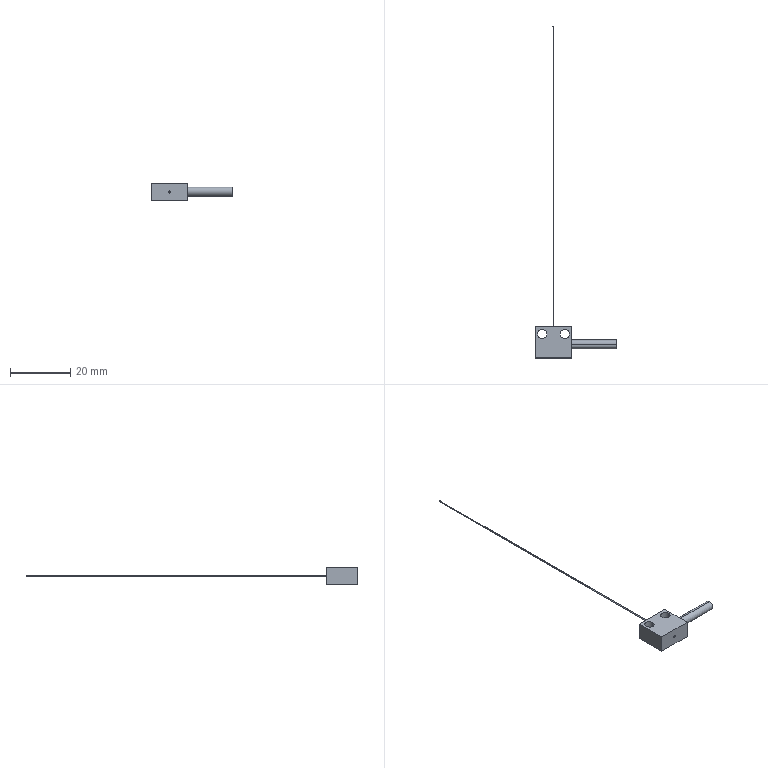Part | STEP file | 11-KEYENCE-PQ0211 | 2 solids | 19 faces | box 27 x 110.5 x 5.8 mm | volume 753.155 mm3 | cylinder 10 | plane 9 | commonest cylinder face diameters 3.1 x4 0.318 x2 0.7 x2 3 x2
STEP:
#1=CARTESIAN_POINT('',(6.,110.5,3.059));
#2=VERTEX_POINT('',#1);
#3=CARTESIAN_POINT('',(6.,110.5,2.741));
#4=VERTEX_POINT('',#3);
#5=CARTESIAN_POINT('',(6.,110.5,2.9));
#6=DIRECTION('',(0.,1.,0.));
#7=DIRECTION('',(0.,0.,1.));
#8=AXIS2_PLACEMENT_3D('',#5,#6,#7);
#9=CIRCLE('',#8,0.1588);
#10=EDGE_CURVE('',#2,#4,#9,.T.);
#11=ORIENTED_EDGE('',*,*,#10,.F.);
#12=CARTESIAN_POINT('',(6.,10.5,3.059));
#13=VERTEX_POINT('',#12);
#14=CARTESIAN_POINT('',(6.,110.5,3.059));
#15=DIRECTION('',(0.,-1.,0.));
#16=VECTOR('',#15,1000.);
#17=LINE('',#14,#16);
#18=EDGE_CURVE('',#2,#13,#17,.T.);
#19=ORIENTED_EDGE('',*,*,#18,.T.);
#20=CARTESIAN_POINT('',(6.,10.5,2.741));
#21=VERTEX_POINT('',#20);
#22=CARTESIAN_POINT('',(6.,10.5,2.9));
#23=DIRECTION('',(0.,1.,0.));
#24=DIRECTION('',(0.,0.,1.));
#25=AXIS2_PLACEMENT_3D('',#22,#23,#24);
#26=CIRCLE('',#25,0.1588);
#27=EDGE_CURVE('',#13,#21,#26,.T.);
#28=ORIENTED_EDGE('',*,*,#27,.T.);
#29=CARTESIAN_POINT('',(6.,110.5,2.741));
#30=DIRECTION('',(0.,-1.,0.));
#31=VECTOR('',#30,1000.);
#32=LINE('',#29,#31);
#33=EDGE_CURVE('',#4,#21,#32,.T.);
#34=ORIENTED_EDGE('',*,*,#33,.F.);
#35=EDGE_LOOP('',(#11,#19,#28,#34));
#36=FACE_OUTER_BOUND('',#35,.T.);
#37=CARTESIAN_POINT('',(6.,110.5,2.9));
#38=DIRECTION('',(0.,-1.,0.));
#39=DIRECTION('',(0.,0.,-1.));
#40=AXIS2_PLACEMENT_3D('',#37,#38,#39);
#41=CYLINDRICAL_SURFACE('',#40,0.1588);
#42=ADVANCED_FACE('',(#36),#41,.T.);
#43=ORIENTED_EDGE('',*,*,#18,.F.);
#44=CARTESIAN_POINT('',(6.,110.5,2.9));
#45=DIRECTION('',(0.,1.,0.));
#46=DIRECTION('',(0.,0.,1.));
#47=AXIS2_PLACEMENT_3D('',#44,#45,#46);
#48=CIRCLE('',#47,0.1588);
#49=EDGE_CURVE('',#4,#2,#48,.T.);
#50=ORIENTED_EDGE('',*,*,#49,.F.);
#51=ORIENTED_EDGE('',*,*,#33,.T.);
#52=CARTESIAN_POINT('',(6.,10.5,2.9));
#53=DIRECTION('',(0.,1.,0.));
#54=DIRECTION('',(0.,0.,1.));
#55=AXIS2_PLACEMENT_3D('',#52,#53,#54);
#56=CIRCLE('',#55,0.1588);
#57=EDGE_CURVE('',#21,#13,#56,.T.);
#58=ORIENTED_EDGE('',*,*,#57,.T.);
#59=EDGE_LOOP('',(#43,#50,#51,#58));
#60=FACE_OUTER_BOUND('',#59,.T.);
#61=CARTESIAN_POINT('',(6.,110.5,2.9));
#62=DIRECTION('',(0.,-1.,0.));
#63=DIRECTION('',(0.,0.,-1.));
#64=AXIS2_PLACEMENT_3D('',#61,#62,#63);
#65=CYLINDRICAL_SURFACE('',#64,0.1588);
#66=ADVANCED_FACE('',(#60),#65,.T.);
#67=ORIENTED_EDGE('',*,*,#49,.T.);
#68=ORIENTED_EDGE('',*,*,#10,.T.);
#69=EDGE_LOOP('',(#67,#68));
#70=FACE_OUTER_BOUND('',#69,.T.);
#71=CARTESIAN_POINT('',(6.,110.5,2.9));
#72=DIRECTION('',(0.,1.,0.));
#73=DIRECTION('',(0.,0.,1.));
#74=AXIS2_PLACEMENT_3D('',#71,#72,#73);
#75=PLANE('',#74);
#76=ADVANCED_FACE('',(#70),#75,.T.);
#77=ORIENTED_EDGE('',*,*,#57,.F.);
#78=ORIENTED_EDGE('',*,*,#27,.F.);
#79=EDGE_LOOP('',(#77,#78));
#80=FACE_OUTER_BOUND('',#79,.T.);
#81=CARTESIAN_POINT('',(6.,10.5,2.9));
#82=DIRECTION('',(0.,1.,0.));
#83=DIRECTION('',(0.,0.,1.));
#84=AXIS2_PLACEMENT_3D('',#81,#82,#83);
#85=PLANE('',#84);
#86=ADVANCED_FACE('',(#80),#85,.F.);
#87=CLOSED_SHELL('',(#42,#66,#76,#86));
#88=MANIFOLD_SOLID_BREP('',#87);
#89=CARTESIAN_POINT('',(6.,0.,2.55));
#90=VERTEX_POINT('',#89);
#91=CARTESIAN_POINT('',(6.,0.,3.25));
#92=VERTEX_POINT('',#91);
#93=CARTESIAN_POINT('',(6.,0.,2.9));
#94=DIRECTION('',(0.,1.,0.));
#95=DIRECTION('',(0.,0.,1.));
#96=AXIS2_PLACEMENT_3D('',#93,#94,#95);
#97=CIRCLE('',#96,0.35);
#98=EDGE_CURVE('',#90,#92,#97,.T.);
#99=ORIENTED_EDGE('',*,*,#98,.F.);
#100=CARTESIAN_POINT('',(6.,10.5,2.55));
#101=VERTEX_POINT('',#100);
#102=CARTESIAN_POINT('',(6.,10.5,2.55));
#103=DIRECTION('',(0.,1.,0.));
#104=VECTOR('',#103,1000.);
#105=LINE('',#102,#104);
#106=EDGE_CURVE('',#90,#101,#105,.T.);
#107=ORIENTED_EDGE('',*,*,#106,.T.);
#108=CARTESIAN_POINT('',(6.,10.5,3.25));
#109=VERTEX_POINT('',#108);
#110=CARTESIAN_POINT('',(6.,10.5,2.9));
#111=DIRECTION('',(0.,1.,0.));
#112=DIRECTION('',(0.,0.,1.));
#113=AXIS2_PLACEMENT_3D('',#110,#111,#112);
#114=CIRCLE('',#113,0.35);
#115=EDGE_CURVE('',#101,#109,#114,.T.);
#116=ORIENTED_EDGE('',*,*,#115,.T.);
#117=CARTESIAN_POINT('',(6.,10.5,3.25));
#118=DIRECTION('',(0.,1.,0.));
#119=VECTOR('',#118,1000.);
#120=LINE('',#117,#119);
#121=EDGE_CURVE('',#92,#109,#120,.T.);
#122=ORIENTED_EDGE('',*,*,#121,.F.);
#123=EDGE_LOOP('',(#99,#107,#116,#122));
#124=FACE_OUTER_BOUND('',#123,.T.);
#125=CARTESIAN_POINT('',(6.,10.5,2.9));
#126=DIRECTION('',(0.,1.,0.));
#127=DIRECTION('',(0.,0.,1.));
#128=AXIS2_PLACEMENT_3D('',#125,#126,#127);
#129=CYLINDRICAL_SURFACE('',#128,0.35);
#130=ADVANCED_FACE('',(#124),#129,.F.);
#131=CARTESIAN_POINT('',(0.7,8.,0.));
#132=VERTEX_POINT('',#131);
#133=CARTESIAN_POINT('',(3.8,8.,0.));
#134=VERTEX_POINT('',#133);
#135=CARTESIAN_POINT('',(2.25,8.,0.));
#136=DIRECTION('',(0.,0.,1.));
#137=DIRECTION('',(1.,0.,0.));
#138=AXIS2_PLACEMENT_3D('',#135,#136,#137);
#139=CIRCLE('',#138,1.55);
#140=EDGE_CURVE('',#132,#134,#139,.T.);
#141=ORIENTED_EDGE('',*,*,#140,.F.);
#142=CARTESIAN_POINT('',(0.7,8.,5.8));
#143=VERTEX_POINT('',#142);
#144=CARTESIAN_POINT('',(0.7,8.,5.8));
#145=DIRECTION('',(0.,0.,1.));
#146=VECTOR('',#145,1000.);
#147=LINE('',#144,#146);
#148=EDGE_CURVE('',#132,#143,#147,.T.);
#149=ORIENTED_EDGE('',*,*,#148,.T.);
#150=CARTESIAN_POINT('',(3.8,8.,5.8));
#151=VERTEX_POINT('',#150);
#152=CARTESIAN_POINT('',(2.25,8.,5.8));
#153=DIRECTION('',(0.,0.,1.));
#154=DIRECTION('',(1.,0.,0.));
#155=AXIS2_PLACEMENT_3D('',#152,#153,#154);
#156=CIRCLE('',#155,1.55);
#157=EDGE_CURVE('',#143,#151,#156,.T.);
#158=ORIENTED_EDGE('',*,*,#157,.T.);
#159=CARTESIAN_POINT('',(3.8,8.,5.8));
#160=DIRECTION('',(0.,0.,1.));
#161=VECTOR('',#160,1000.);
#162=LINE('',#159,#161);
#163=EDGE_CURVE('',#134,#151,#162,.T.);
#164=ORIENTED_EDGE('',*,*,#163,.F.);
#165=EDGE_LOOP('',(#141,#149,#158,#164));
#166=FACE_OUTER_BOUND('',#165,.T.);
#167=CARTESIAN_POINT('',(2.25,8.,5.8));
#168=DIRECTION('',(0.,0.,1.));
#169=DIRECTION('',(1.,0.,0.));
#170=AXIS2_PLACEMENT_3D('',#167,#168,#169);
#171=CYLINDRICAL_SURFACE('',#170,1.55);
#172=ADVANCED_FACE('',(#166),#171,.F.);
#173=CARTESIAN_POINT('',(8.2,8.,0.));
#174=VERTEX_POINT('',#173);
#175=CARTESIAN_POINT('',(11.3,8.,0.));
#176=VERTEX_POINT('',#175);
#177=CARTESIAN_POINT('',(9.75,8.,0.));
#178=DIRECTION('',(0.,0.,1.));
#179=DIRECTION('',(1.,0.,0.));
#180=AXIS2_PLACEMENT_3D('',#177,#178,#179);
#181=CIRCLE('',#180,1.55);
#182=EDGE_CURVE('',#174,#176,#181,.T.);
#183=ORIENTED_EDGE('',*,*,#182,.F.);
#184=CARTESIAN_POINT('',(8.2,8.,5.8));
#185=VERTEX_POINT('',#184);
#186=CARTESIAN_POINT('',(8.2,8.,5.8));
#187=DIRECTION('',(0.,0.,1.));
#188=VECTOR('',#187,1000.);
#189=LINE('',#186,#188);
#190=EDGE_CURVE('',#174,#185,#189,.T.);
#191=ORIENTED_EDGE('',*,*,#190,.T.);
#192=CARTESIAN_POINT('',(11.3,8.,5.8));
#193=VERTEX_POINT('',#192);
#194=CARTESIAN_POINT('',(9.75,8.,5.8));
#195=DIRECTION('',(0.,0.,1.));
#196=DIRECTION('',(1.,0.,0.));
#197=AXIS2_PLACEMENT_3D('',#194,#195,#196);
#198=CIRCLE('',#197,1.55);
#199=EDGE_CURVE('',#185,#193,#198,.T.);
#200=ORIENTED_EDGE('',*,*,#199,.T.);
#201=CARTESIAN_POINT('',(11.3,8.,5.8));
#202=DIRECTION('',(0.,0.,1.));
#203=VECTOR('',#202,1000.);
#204=LINE('',#201,#203);
#205=EDGE_CURVE('',#176,#193,#204,.T.);
#206=ORIENTED_EDGE('',*,*,#205,.F.);
#207=EDGE_LOOP('',(#183,#191,#200,#206));
#208=FACE_OUTER_BOUND('',#207,.T.);
#209=CARTESIAN_POINT('',(9.75,8.,5.8));
#210=DIRECTION('',(0.,0.,1.));
#211=DIRECTION('',(1.,0.,0.));
#212=AXIS2_PLACEMENT_3D('',#209,#210,#211);
#213=CYLINDRICAL_SURFACE('',#212,1.55);
#214=ADVANCED_FACE('',(#208),#213,.F.);
#215=CARTESIAN_POINT('',(27.,4.5,1.5));
#216=VERTEX_POINT('',#215);
#217=CARTESIAN_POINT('',(27.,4.5,4.5));
#218=VERTEX_POINT('',#217);
#219=CARTESIAN_POINT('',(27.,4.5,3.));
#220=DIRECTION('',(1.,0.,0.));
#221=DIRECTION('',(0.,0.,-1.));
#222=AXIS2_PLACEMENT_3D('',#219,#220,#221);
#223=CIRCLE('',#222,1.5);
#224=EDGE_CURVE('',#216,#218,#223,.T.);
#225=ORIENTED_EDGE('',*,*,#224,.F.);
#226=CARTESIAN_POINT('',(12.,4.5,1.5));
#227=VERTEX_POINT('',#226);
#228=CARTESIAN_POINT('',(27.,4.5,1.5));
#229=DIRECTION('',(-1.,0.,0.));
#230=VECTOR('',#229,1000.);
#231=LINE('',#228,#230);
#232=EDGE_CURVE('',#216,#227,#231,.T.);
#233=ORIENTED_EDGE('',*,*,#232,.T.);
#234=CARTESIAN_POINT('',(12.,4.5,4.5));
#235=VERTEX_POINT('',#234);
#236=CARTESIAN_POINT('',(12.,4.5,3.));
#237=DIRECTION('',(1.,0.,0.));
#238=DIRECTION('',(0.,0.,1.));
#239=AXIS2_PLACEMENT_3D('',#236,#237,#238);
#240=CIRCLE('',#239,1.5);
#241=EDGE_CURVE('',#227,#235,#240,.T.);
#242=ORIENTED_EDGE('',*,*,#241,.T.);
#243=CARTESIAN_POINT('',(27.,4.5,4.5));
#244=DIRECTION('',(-1.,0.,0.));
#245=VECTOR('',#244,1000.);
#246=LINE('',#243,#245);
#247=EDGE_CURVE('',#218,#235,#246,.T.);
#248=ORIENTED_EDGE('',*,*,#247,.F.);
#249=EDGE_LOOP('',(#225,#233,#242,#248));
#250=FACE_OUTER_BOUND('',#249,.T.);
#251=CARTESIAN_POINT('',(27.,4.5,3.));
#252=DIRECTION('',(-1.,0.,0.));
#253=DIRECTION('',(0.,0.,1.));
#254=AXIS2_PLACEMENT_3D('',#251,#252,#253);
#255=CYLINDRICAL_SURFACE('',#254,1.5);
#256=ADVANCED_FACE('',(#250),#255,.T.);
#257=CARTESIAN_POINT('',(12.,0.,0.));
#258=VERTEX_POINT('',#257);
#259=CARTESIAN_POINT('',(12.,10.5,0.));
#260=VERTEX_POINT('',#259);
#261=CARTESIAN_POINT('',(12.,0.,0.));
#262=DIRECTION('',(0.,1.,0.));
#263=VECTOR('',#262,1000.);
#264=LINE('',#261,#263);
#265=EDGE_CURVE('',#258,#260,#264,.T.);
#266=ORIENTED_EDGE('',*,*,#265,.T.);
#267=CARTESIAN_POINT('',(12.,10.5,5.8));
#268=VERTEX_POINT('',#267);
#269=CARTESIAN_POINT('',(12.,10.5,5.8));
#270=DIRECTION('',(0.,0.,-1.));
#271=VECTOR('',#270,1000.);
#272=LINE('',#269,#271);
#273=EDGE_CURVE('',#268,#260,#272,.T.);
#274=ORIENTED_EDGE('',*,*,#273,.F.);
#275=CARTESIAN_POINT('',(12.,0.,5.8));
#276=VERTEX_POINT('',#275);
#277=CARTESIAN_POINT('',(12.,0.,5.8));
#278=DIRECTION('',(0.,1.,0.));
#279=VECTOR('',#278,1000.);
#280=LINE('',#277,#279);
#281=EDGE_CURVE('',#276,#268,#280,.T.);
#282=ORIENTED_EDGE('',*,*,#281,.F.);
#283=CARTESIAN_POINT('',(12.,0.,5.8));
#284=DIRECTION('',(0.,0.,-1.));
#285=VECTOR('',#284,1000.);
#286=LINE('',#283,#285);
#287=EDGE_CURVE('',#276,#258,#286,.T.);
#288=ORIENTED_EDGE('',*,*,#287,.T.);
#289=EDGE_LOOP('',(#266,#274,#282,#288));
#290=FACE_OUTER_BOUND('',#289,.T.);
#291=CARTESIAN_POINT('',(12.,4.5,3.));
#292=DIRECTION('',(1.,0.,0.));
#293=DIRECTION('',(0.,0.,1.));
#294=AXIS2_PLACEMENT_3D('',#291,#292,#293);
#295=CIRCLE('',#294,1.5);
#296=EDGE_CURVE('',#235,#227,#295,.T.);
#297=ORIENTED_EDGE('',*,*,#296,.F.);
#298=ORIENTED_EDGE('',*,*,#241,.F.);
#299=EDGE_LOOP('',(#297,#298));
#300=FACE_BOUND('',#299,.T.);
#301=CARTESIAN_POINT('',(12.,0.,5.8));
#302=DIRECTION('',(-1.,0.,0.));
#303=DIRECTION('',(0.,0.,1.));
#304=AXIS2_PLACEMENT_3D('',#301,#302,#303);
#305=PLANE('',#304);
#306=ADVANCED_FACE('',(#290,#300),#305,.F.);
#307=CARTESIAN_POINT('',(0.,10.5,0.));
#308=VERTEX_POINT('',#307);
#309=CARTESIAN_POINT('',(0.,0.,0.));
#310=VERTEX_POINT('',#309);
#311=CARTESIAN_POINT('',(0.,0.,0.));
#312=DIRECTION('',(0.,-1.,0.));
#313=VECTOR('',#312,1000.);
#314=LINE('',#311,#313);
#315=EDGE_CURVE('',#308,#310,#314,.T.);
#316=ORIENTED_EDGE('',*,*,#315,.T.);
#317=CARTESIAN_POINT('',(0.,0.,5.8));
#318=VERTEX_POINT('',#317);
#319=CARTESIAN_POINT('',(0.,0.,5.8));
#320=DIRECTION('',(0.,0.,-1.));
#321=VECTOR('',#320,1000.);
#322=LINE('',#319,#321);
#323=EDGE_CURVE('',#318,#310,#322,.T.);
#324=ORIENTED_EDGE('',*,*,#323,.F.);
#325=CARTESIAN_POINT('',(0.,10.5,5.8));
#326=VERTEX_POINT('',#325);
#327=CARTESIAN_POINT('',(0.,0.,5.8));
#328=DIRECTION('',(0.,-1.,0.));
#329=VECTOR('',#328,1000.);
#330=LINE('',#327,#329);
#331=EDGE_CURVE('',#326,#318,#330,.T.);
#332=ORIENTED_EDGE('',*,*,#331,.F.);
#333=CARTESIAN_POINT('',(0.,10.5,5.8));
#334=DIRECTION('',(0.,0.,-1.));
#335=VECTOR('',#334,1000.);
#336=LINE('',#333,#335);
#337=EDGE_CURVE('',#326,#308,#336,.T.);
#338=ORIENTED_EDGE('',*,*,#337,.T.);
#339=EDGE_LOOP('',(#316,#324,#332,#338));
#340=FACE_OUTER_BOUND('',#339,.T.);
#341=CARTESIAN_POINT('',(0.,0.,5.8));
#342=DIRECTION('',(1.,0.,0.));
#343=DIRECTION('',(0.,0.,-1.));
#344=AXIS2_PLACEMENT_3D('',#341,#342,#343);
#345=PLANE('',#344);
#346=ADVANCED_FACE('',(#340),#345,.F.);
#347=CARTESIAN_POINT('',(6.,0.,2.9));
#348=DIRECTION('',(0.,1.,0.));
#349=DIRECTION('',(0.,0.,1.));
#350=AXIS2_PLACEMENT_3D('',#347,#348,#349);
#351=CIRCLE('',#350,0.35);
#352=EDGE_CURVE('',#92,#90,#351,.T.);
#353=ORIENTED_EDGE('',*,*,#352,.T.);
#354=ORIENTED_EDGE('',*,*,#98,.T.);
#355=EDGE_LOOP('',(#353,#354));
#356=FACE_BOUND('',#355,.T.);
#357=CARTESIAN_POINT('',(0.,0.,0.));
#358=DIRECTION('',(1.,0.,0.));
#359=VECTOR('',#358,1000.);
#360=LINE('',#357,#359);
#361=EDGE_CURVE('',#310,#258,#360,.T.);
#362=ORIENTED_EDGE('',*,*,#361,.T.);
#363=ORIENTED_EDGE('',*,*,#287,.F.);
#364=CARTESIAN_POINT('',(0.,0.,5.8));
#365=DIRECTION('',(1.,0.,0.));
#366=VECTOR('',#365,1000.);
#367=LINE('',#364,#366);
#368=EDGE_CURVE('',#318,#276,#367,.T.);
#369=ORIENTED_EDGE('',*,*,#368,.F.);
#370=ORIENTED_EDGE('',*,*,#323,.T.);
#371=EDGE_LOOP('',(#362,#363,#369,#370));
#372=FACE_OUTER_BOUND('',#371,.T.);
#373=CARTESIAN_POINT('',(0.,0.,5.8));
#374=DIRECTION('',(0.,1.,0.));
#375=DIRECTION('',(0.,0.,1.));
#376=AXIS2_PLACEMENT_3D('',#373,#374,#375);
#377=PLANE('',#376);
#378=ADVANCED_FACE('',(#356,#372),#377,.F.);
#379=CARTESIAN_POINT('',(6.,10.5,2.9));
#380=DIRECTION('',(0.,1.,0.));
#381=DIRECTION('',(0.,0.,1.));
#382=AXIS2_PLACEMENT_3D('',#379,#380,#381);
#383=CIRCLE('',#382,0.35);
#384=EDGE_CURVE('',#109,#101,#383,.T.);
#385=ORIENTED_EDGE('',*,*,#384,.F.);
#386=ORIENTED_EDGE('',*,*,#115,.F.);
#387=EDGE_LOOP('',(#385,#386));
#388=FACE_BOUND('',#387,.T.);
#389=CARTESIAN_POINT('',(0.,10.5,0.));
#390=DIRECTION('',(-1.,0.,0.));
#391=VECTOR('',#390,1000.);
#392=LINE('',#389,#391);
#393=EDGE_CURVE('',#260,#308,#392,.T.);
#394=ORIENTED_EDGE('',*,*,#393,.T.);
#395=ORIENTED_EDGE('',*,*,#337,.F.);
#396=CARTESIAN_POINT('',(0.,10.5,5.8));
#397=DIRECTION('',(-1.,0.,0.));
#398=VECTOR('',#397,1000.);
#399=LINE('',#396,#398);
#400=EDGE_CURVE('',#268,#326,#399,.T.);
#401=ORIENTED_EDGE('',*,*,#400,.F.);
#402=ORIENTED_EDGE('',*,*,#273,.T.);
#403=EDGE_LOOP('',(#394,#395,#401,#402));
#404=FACE_OUTER_BOUND('',#403,.T.);
#405=CARTESIAN_POINT('',(0.,10.5,5.8));
#406=DIRECTION('',(0.,-1.,0.));
#407=DIRECTION('',(0.,0.,-1.));
#408=AXIS2_PLACEMENT_3D('',#405,#406,#407);
#409=PLANE('',#408);
#410=ADVANCED_FACE('',(#388,#404),#409,.F.);
#411=CARTESIAN_POINT('',(2.25,8.,5.8));
#412=DIRECTION('',(0.,0.,1.));
#413=DIRECTION('',(1.,0.,0.));
#414=AXIS2_PLACEMENT_3D('',#411,#412,#413);
#415=CIRCLE('',#414,1.55);
#416=EDGE_CURVE('',#151,#143,#415,.T.);
#417=ORIENTED_EDGE('',*,*,#416,.F.);
#418=ORIENTED_EDGE('',*,*,#157,.F.);
#419=EDGE_LOOP('',(#417,#418));
#420=FACE_BOUND('',#419,.T.);
#421=CARTESIAN_POINT('',(9.75,8.,5.8));
#422=DIRECTION('',(0.,0.,1.));
#423=DIRECTION('',(1.,0.,0.));
#424=AXIS2_PLACEMENT_3D('',#421,#422,#423);
#425=CIRCLE('',#424,1.55);
#426=EDGE_CURVE('',#193,#185,#425,.T.);
#427=ORIENTED_EDGE('',*,*,#426,.F.);
#428=ORIENTED_EDGE('',*,*,#199,.F.);
#429=EDGE_LOOP('',(#427,#428));
#430=FACE_BOUND('',#429,.T.);
#431=ORIENTED_EDGE('',*,*,#331,.T.);
#432=ORIENTED_EDGE('',*,*,#368,.T.);
#433=ORIENTED_EDGE('',*,*,#281,.T.);
#434=ORIENTED_EDGE('',*,*,#400,.T.);
#435=EDGE_LOOP('',(#431,#432,#433,#434));
#436=FACE_OUTER_BOUND('',#435,.T.);
#437=CARTESIAN_POINT('',(0.,10.5,5.8));
#438=DIRECTION('',(0.,0.,-1.));
#439=DIRECTION('',(-1.,0.,0.));
#440=AXIS2_PLACEMENT_3D('',#437,#438,#439);
#441=PLANE('',#440);
#442=ADVANCED_FACE('',(#420,#430,#436),#441,.F.);
#443=CARTESIAN_POINT('',(2.25,8.,0.));
#444=DIRECTION('',(0.,0.,1.));
#445=DIRECTION('',(1.,0.,0.));
#446=AXIS2_PLACEMENT_3D('',#443,#444,#445);
#447=CIRCLE('',#446,1.55);
#448=EDGE_CURVE('',#134,#132,#447,.T.);
#449=ORIENTED_EDGE('',*,*,#448,.T.);
#450=ORIENTED_EDGE('',*,*,#140,.T.);
#451=EDGE_LOOP('',(#449,#450));
#452=FACE_BOUND('',#451,.T.);
#453=CARTESIAN_POINT('',(9.75,8.,0.));
#454=DIRECTION('',(0.,0.,1.));
#455=DIRECTION('',(1.,0.,0.));
#456=AXIS2_PLACEMENT_3D('',#453,#454,#455);
#457=CIRCLE('',#456,1.55);
#458=EDGE_CURVE('',#176,#174,#457,.T.);
#459=ORIENTED_EDGE('',*,*,#458,.T.);
#460=ORIENTED_EDGE('',*,*,#182,.T.);
#461=EDGE_LOOP('',(#459,#460));
#462=FACE_BOUND('',#461,.T.);
#463=ORIENTED_EDGE('',*,*,#315,.F.);
#464=ORIENTED_EDGE('',*,*,#393,.F.);
#465=ORIENTED_EDGE('',*,*,#265,.F.);
#466=ORIENTED_EDGE('',*,*,#361,.F.);
#467=EDGE_LOOP('',(#463,#464,#465,#466));
#468=FACE_OUTER_BOUND('',#467,.T.);
#469=CARTESIAN_POINT('',(0.,10.5,0.));
#470=DIRECTION('',(0.,0.,-1.));
#471=DIRECTION('',(-1.,0.,0.));
#472=AXIS2_PLACEMENT_3D('',#469,#470,#471);
#473=PLANE('',#472);
#474=ADVANCED_FACE('',(#452,#462,#468),#473,.T.);
#475=ORIENTED_EDGE('',*,*,#232,.F.);
#476=CARTESIAN_POINT('',(27.,4.5,3.));
#477=DIRECTION('',(1.,0.,0.));
#478=DIRECTION('',(0.,0.,-1.));
#479=AXIS2_PLACEMENT_3D('',#476,#477,#478);
#480=CIRCLE('',#479,1.5);
#481=EDGE_CURVE('',#218,#216,#480,.T.);
#482=ORIENTED_EDGE('',*,*,#481,.F.);
#483=ORIENTED_EDGE('',*,*,#247,.T.);
#484=ORIENTED_EDGE('',*,*,#296,.T.);
#485=EDGE_LOOP('',(#475,#482,#483,#484));
#486=FACE_OUTER_BOUND('',#485,.T.);
#487=CARTESIAN_POINT('',(27.,4.5,3.));
#488=DIRECTION('',(-1.,0.,0.));
#489=DIRECTION('',(0.,0.,1.));
#490=AXIS2_PLACEMENT_3D('',#487,#488,#489);
#491=CYLINDRICAL_SURFACE('',#490,1.5);
#492=ADVANCED_FACE('',(#486),#491,.T.);
#493=ORIENTED_EDGE('',*,*,#481,.T.);
#494=ORIENTED_EDGE('',*,*,#224,.T.);
#495=EDGE_LOOP('',(#493,#494));
#496=FACE_OUTER_BOUND('',#495,.T.);
#497=CARTESIAN_POINT('',(27.,4.5,3.));
#498=DIRECTION('',(1.,0.,0.));
#499=DIRECTION('',(0.,0.,-1.));
#500=AXIS2_PLACEMENT_3D('',#497,#498,#499);
#501=PLANE('',#500);
#502=ADVANCED_FACE('',(#496),#501,.T.);
#503=ORIENTED_EDGE('',*,*,#190,.F.);
#504=ORIENTED_EDGE('',*,*,#458,.F.);
#505=ORIENTED_EDGE('',*,*,#205,.T.);
#506=ORIENTED_EDGE('',*,*,#426,.T.);
#507=EDGE_LOOP('',(#503,#504,#505,#506));
#508=FACE_OUTER_BOUND('',#507,.T.);
#509=CARTESIAN_POINT('',(9.75,8.,5.8));
#510=DIRECTION('',(0.,0.,1.));
#511=DIRECTION('',(1.,0.,0.));
#512=AXIS2_PLACEMENT_3D('',#509,#510,#511);
#513=CYLINDRICAL_SURFACE('',#512,1.55);
#514=ADVANCED_FACE('',(#508),#513,.F.);
#515=ORIENTED_EDGE('',*,*,#148,.F.);
#516=ORIENTED_EDGE('',*,*,#448,.F.);
#517=ORIENTED_EDGE('',*,*,#163,.T.);
#518=ORIENTED_EDGE('',*,*,#416,.T.);
#519=EDGE_LOOP('',(#515,#516,#517,#518));
#520=FACE_OUTER_BOUND('',#519,.T.);
#521=CARTESIAN_POINT('',(2.25,8.,5.8));
#522=DIRECTION('',(0.,0.,1.));
#523=DIRECTION('',(1.,0.,0.));
#524=AXIS2_PLACEMENT_3D('',#521,#522,#523);
#525=CYLINDRICAL_SURFACE('',#524,1.55);
#526=ADVANCED_FACE('',(#520),#525,.F.);
#527=ORIENTED_EDGE('',*,*,#106,.F.);
#528=ORIENTED_EDGE('',*,*,#352,.F.);
#529=ORIENTED_EDGE('',*,*,#121,.T.);
#530=ORIENTED_EDGE('',*,*,#384,.T.);
#531=EDGE_LOOP('',(#527,#528,#529,#530));
#532=FACE_OUTER_BOUND('',#531,.T.);
#533=CARTESIAN_POINT('',(6.,10.5,2.9));
#534=DIRECTION('',(0.,1.,0.));
#535=DIRECTION('',(0.,0.,1.));
#536=AXIS2_PLACEMENT_3D('',#533,#534,#535);
#537=CYLINDRICAL_SURFACE('',#536,0.35);
#538=ADVANCED_FACE('',(#532),#537,.F.);
#539=CLOSED_SHELL('',(#130,#172,#214,#256,#306,#346,#378,#410,#442,#474,#492,#502,#514,#526,#538));
#540=MANIFOLD_SOLID_BREP('',#539);
#541=CARTESIAN_POINT('',(0.,0.,0.));
#542=DIRECTION('',(0.,0.,1.));
#543=DIRECTION('',(1.,0.,0.));
#544=AXIS2_PLACEMENT_3D('',#541,#542,#543);
#545=(LENGTH_UNIT()NAMED_UNIT(*)SI_UNIT(.MILLI.,.METRE.));
#546=UNCERTAINTY_MEASURE_WITH_UNIT(LENGTH_MEASURE(0.00001),#545,'','');
#547=(NAMED_UNIT(*)PLANE_ANGLE_UNIT()SI_UNIT($,.RADIAN.));
#548=(NAMED_UNIT(*)SI_UNIT($,.STERADIAN.)SOLID_ANGLE_UNIT());
#549=(GEOMETRIC_REPRESENTATION_CONTEXT(3)GLOBAL_UNCERTAINTY_ASSIGNED_CONTEXT((#546))GLOBAL_UNIT_ASSIGNED_CONTEXT((#545,#547,#548))REPRESENTATION_CONTEXT('',''));
#550=ADVANCED_BREP_SHAPE_REPRESENTATION('',(#88,#540,#544),#549);